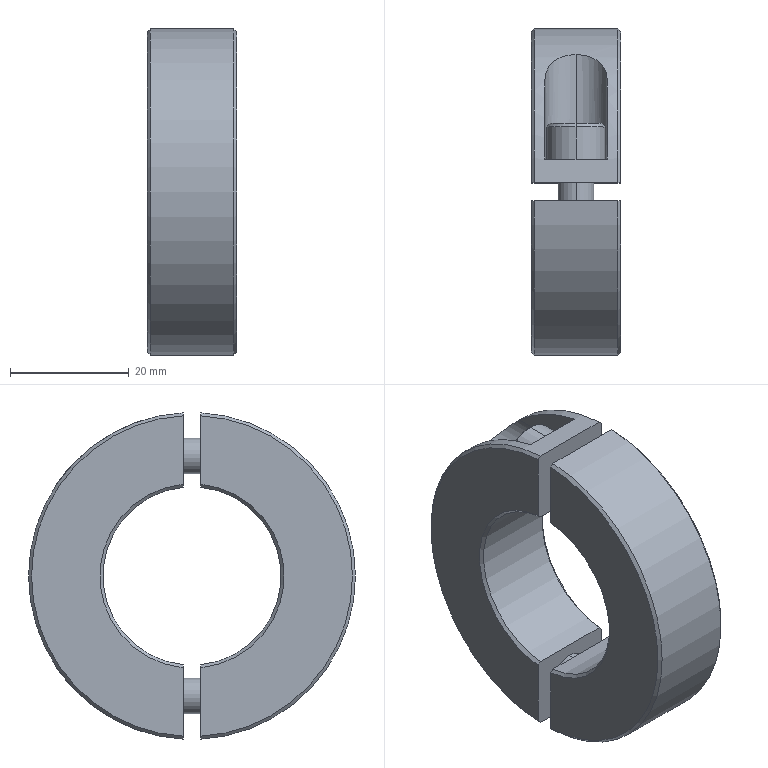Part | STEP file | Split Shaft Collar_ Steel GN 707.2-55-B30-STV11 | 1 solid | 91 faces | box 15 x 55 x 54.918 mm | volume 22142 mm3 | plane 44 | cone 24 | cylinder 23 | commonest cylinder face diameters 4.917 x4 6 x4 6.3 x4 10 x4 10.5 x3 30 x2